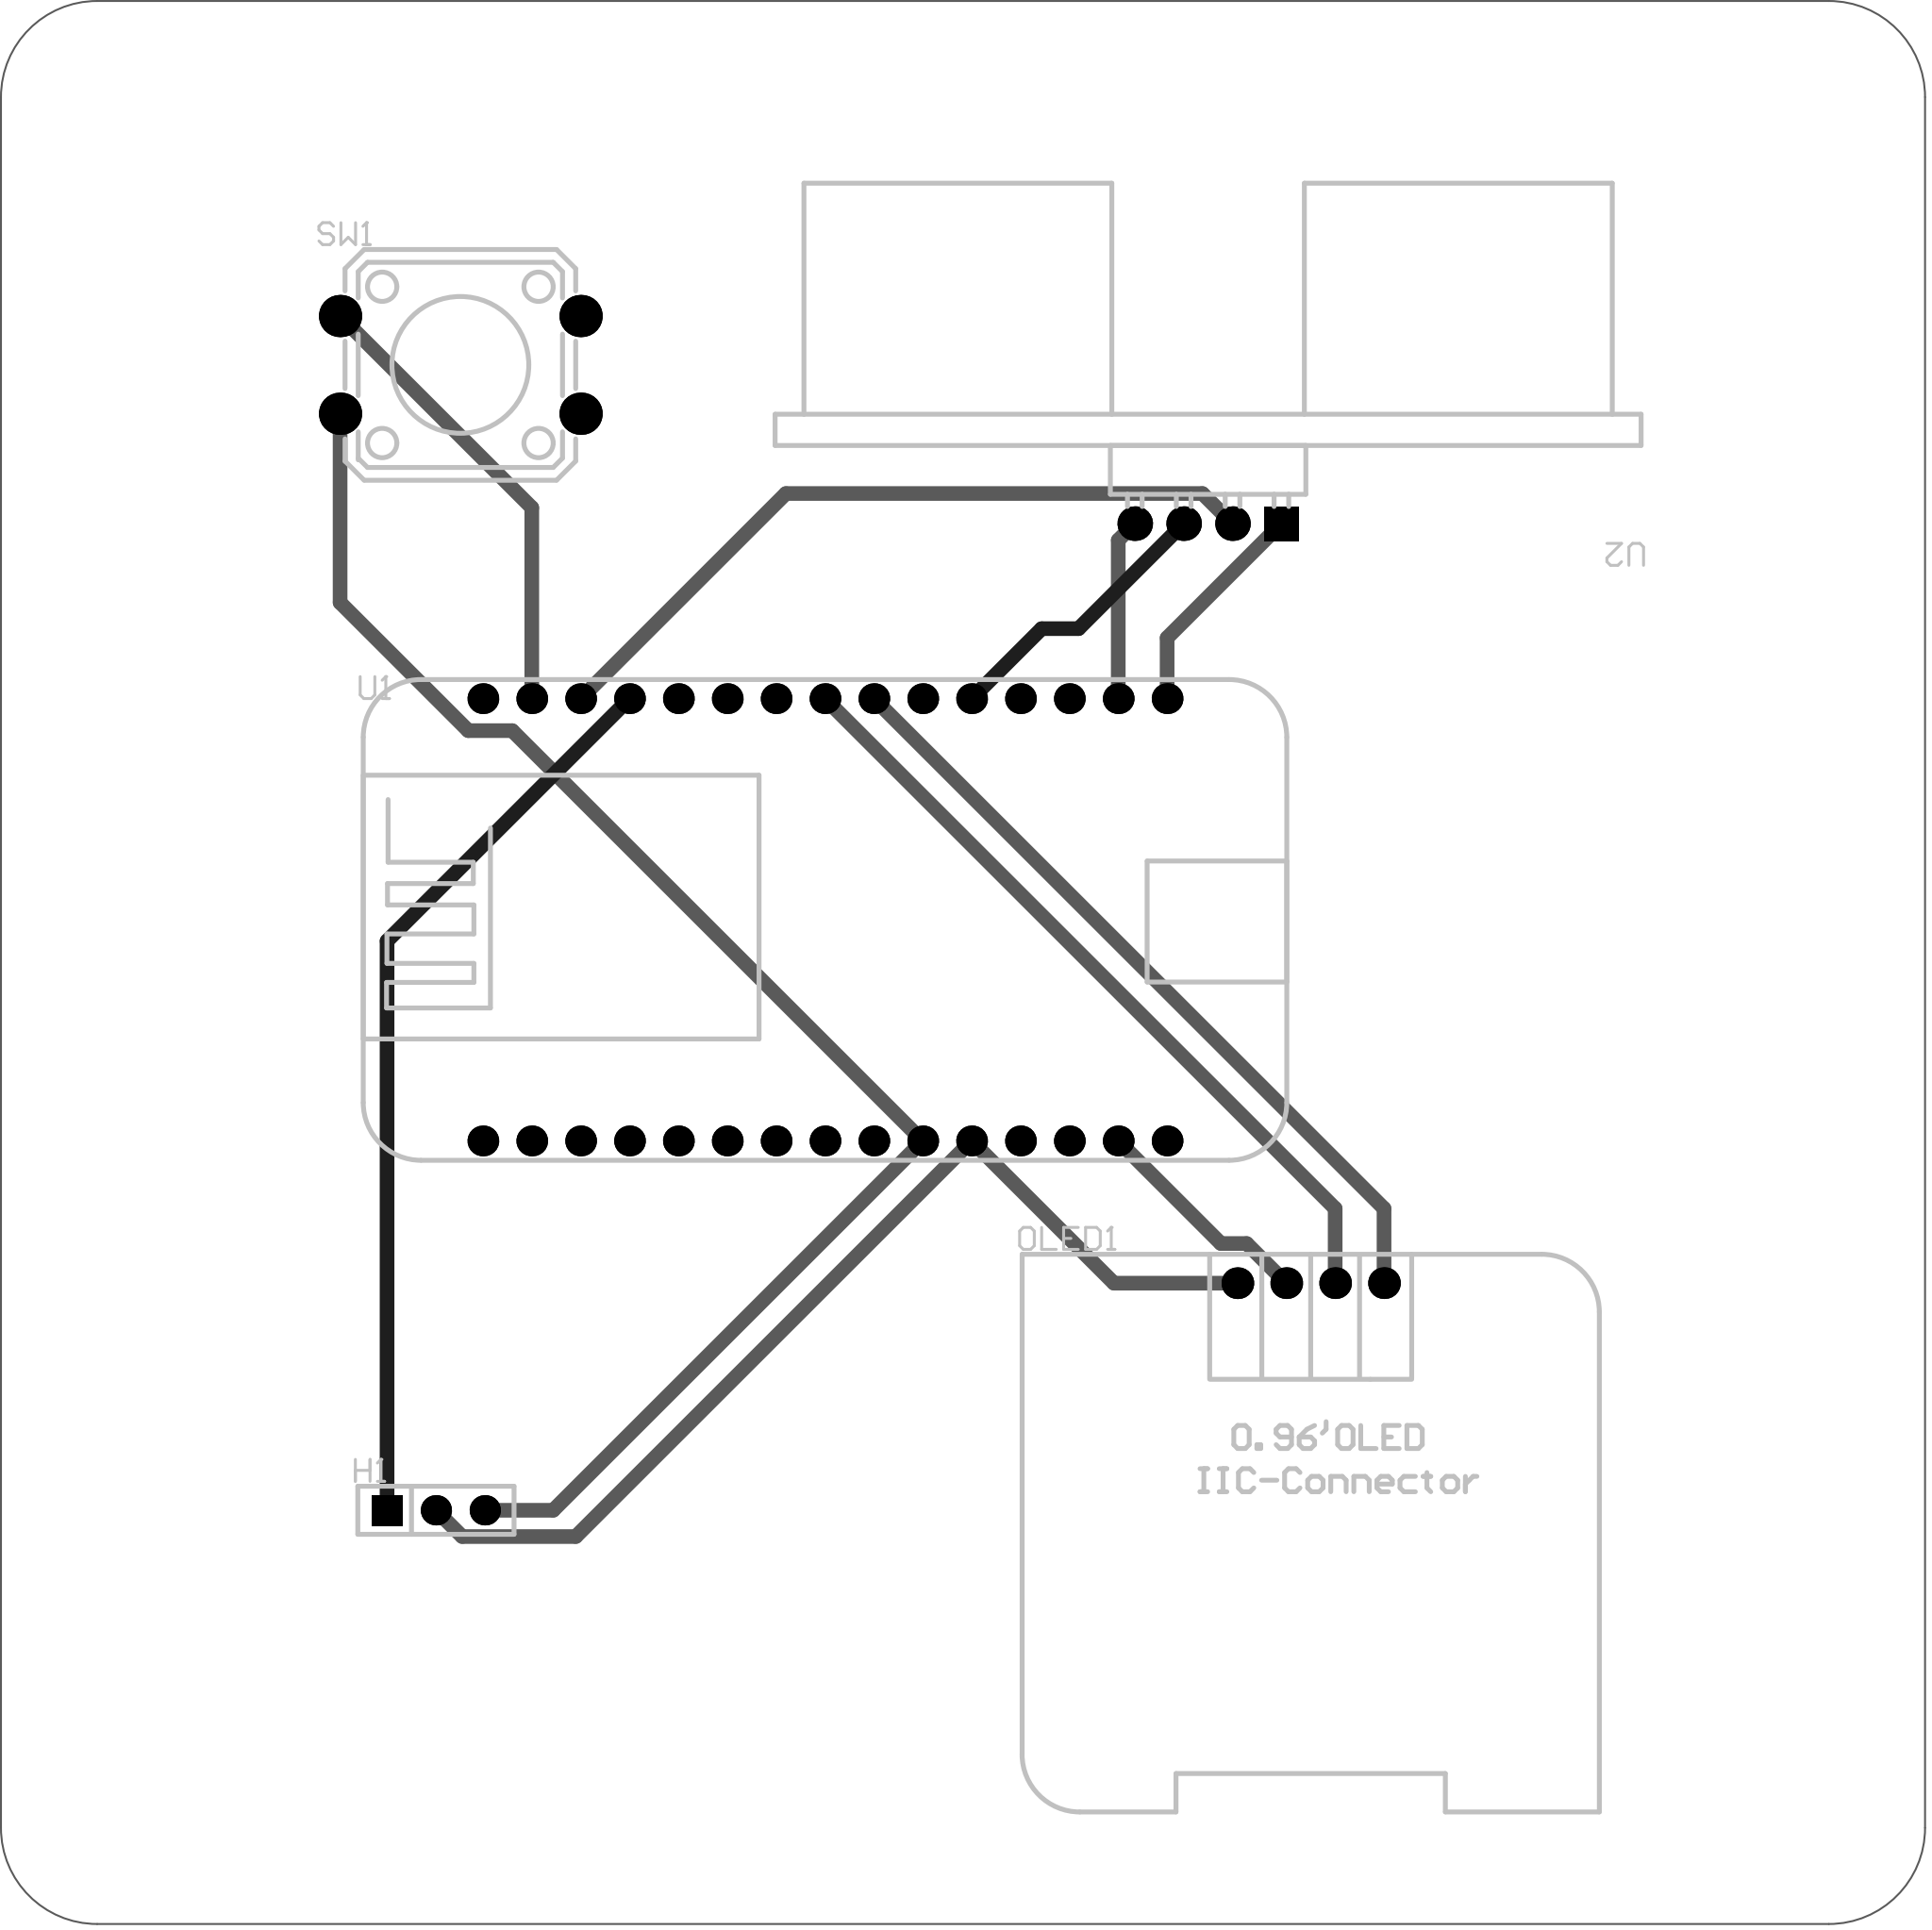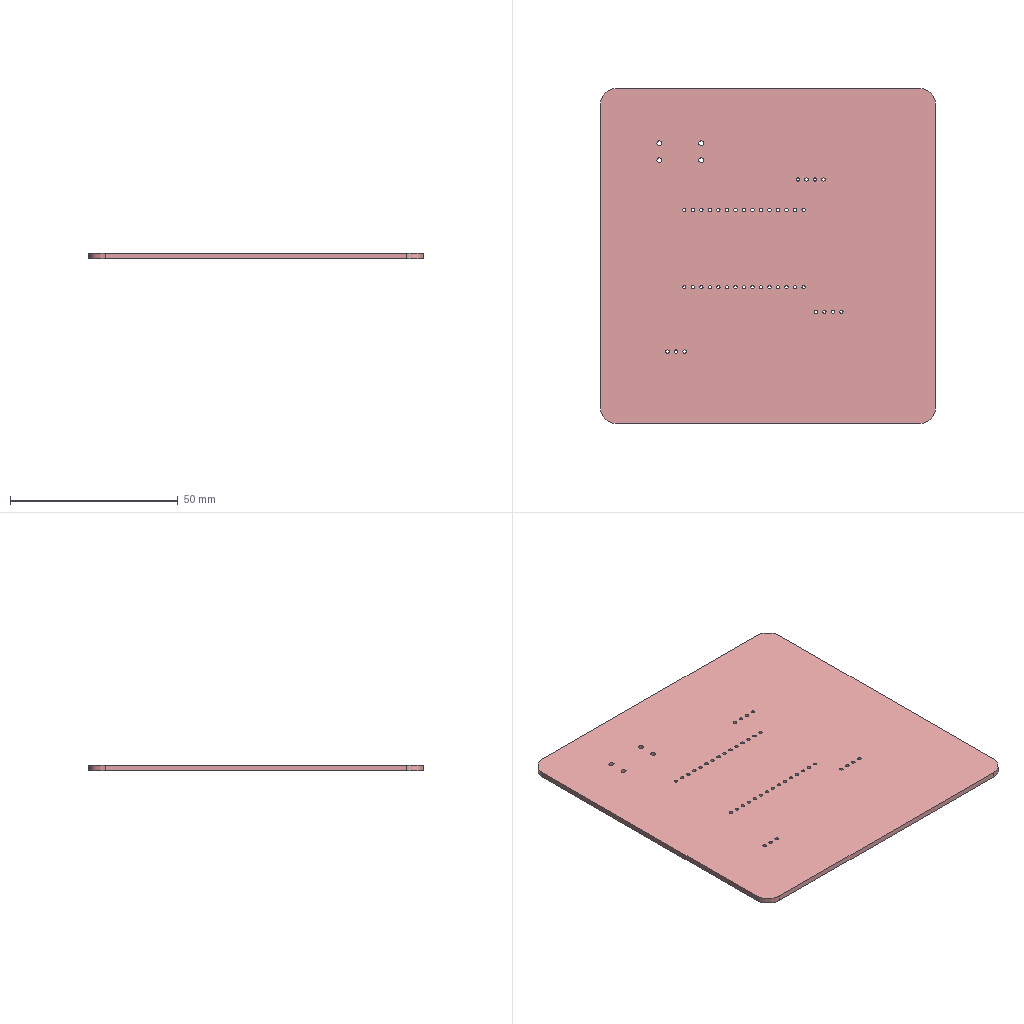Circuit board layout | Altium Designer | box 100 x 100 x 1.6 mm
Layer stack:
# Altium Designer layer stack of  (unit mm; dielectric type: 0 none, 1 core, 2 prepreg, 3 surface material)
index,name,kind,layer,copper_thickness_mm,dielectric_type,dielectric_thickness_mm,dielectric_material,dielectric_constant
0,Top Paste Mask Layer,other,,,,,,
1,Top Silkscreen Layer,other,,,,,,
2,Top Solder Mask Layer,dielectric,,,3,0.01,,3.3
3,Top Layer,copper,Top Layer,0.035,,,,
4,Dielectric1,dielectric,,,3,1.51,FR4,4.5
5,Bottom Layer,copper,Bottom Layer,0.035,,,,
6,Bottom Solder Mask Layer,dielectric,,,3,0.01,,3.3
7,Bottom Silkscreen Layer,other,,,,,,
8,Bottom Paste Mask Layer,other,,,,,,
# drill layer pairs: low layer,high layer
drill_pair,Top Layer,Bottom Layer
Part placement:
Designator,Comment,Layer,Footprint,Center-X(mm),Center-Y(mm),Rotation
U1,STM32F103C8T6-Card,TopLayer,CONN-TH_L53.3-W22.9_STM32F103C8T6-CARD,119.028,128.421,0
OLED1,,TopLayer,0.96OLED_4P,144.272,109.525,0
H1,,TopLayer,HDR-TH_3P-P2.54-V-F,98.806,97.714,0
SW1,Tactile switch, 12*12*6 plastic head, 260G, travel 0.25mm, through-hole,TopLayer,KEY-TH_4P-L12.0-W12.0-P5.00-LS12.5,100.076,157.277,0
U2,HC-SR04,TopLayer,TH_HC-SR04V,138.938,149.022,180
Pad and via stacks:
# Altium Designer via and pad stacks of  (unit mm). Each distinct definition once, with the count of objects using it.
# via: kind,start_layer,end_layer,hole_mm,diameter_mm,mode(0 simple;1 top-mid-bottom;2 full stack),diameter_per_layer,count,example_net
# pad: kind,layer,hole_mm,hole_type(0 round;1 square;2 slot),plating,top_size,top_shape(1 round;2 rect;3 octagon;9 rounded rect),mid_size,bottom_size,mode,footprint,size_per_layer,count,example
pad,Multi-Layer,1,0,plated,1.6x1.6,1,1.6x1.6,1.6x1.6,0,CONN-TH_L53.3-W22.9_STM32F103C8T6-CARD,,30,U1.1
pad,Multi-Layer,1,0,plated,1.65x1.65,1,1.65x1.65,1.65x1.65,0,0.96OLED_4P,,4,OLED1.4
pad,Multi-Layer,1.02,0,plated,1.575x1.575,1,1.575x1.575,1.575x1.575,0,HDR-TH_3P-P2.54-V-F,,2,H1.3
pad,Multi-Layer,1.02,0,plated,1.575x1.575,2,1.575x1.575,1.575x1.575,0,HDR-TH_3P-P2.54-V-F,,1,H1.1
pad,Multi-Layer,1.5,0,plated,2.2x2.2,1,2.2x2.2,2.2x2.2,0,KEY-TH_4P-L12.0-W12.0-P5.00-LS12.5,,4,SW1.1
pad,Multi-Layer,1.001,0,plated,1.8x1.8,1,1.8x1.8,1.8x1.8,0,TH_HC-SR04V,,3,U2.4
pad,Multi-Layer,1.001,0,plated,1.8x1.8,2,1.8x1.8,1.8x1.8,0,TH_HC-SR04V,,1,U2.1
Design rules, without the lines most boards share:
# Altium Designer design rules of  (exported by Altium Designer, unit mm)
# columns: name | kind | enabled | priority | scope1 | scope2 | descriptor | typed fields (field=value)
copperThickness1oz_2 | 2 | enabled | 2 | All | All | Width Constraint (Min=5mil) (Max=100mil) (Preferred=30mil) (All) |
viaSize | 11 | enabled | 1 | All | All | Routing Via (MinHoleWidth=11.811mil) (MaxHoleWidth=248.032mil) (PreferredHoleWidth=12.008mil) (MinWidth=19.685mil) (MaxWidth=393.701mil) (PreferedWidth=24.016mil) (All) | via_min_hole=0.3 via_max_hole=6.3 via_preferred_diameter=0.61 via_preferred_hole=0.305
solderMaskExpansion | 13 | enabled | 2 | All | All | Solder Mask Expansion (Expansion =2.008mil) (All) | expansion=0.051